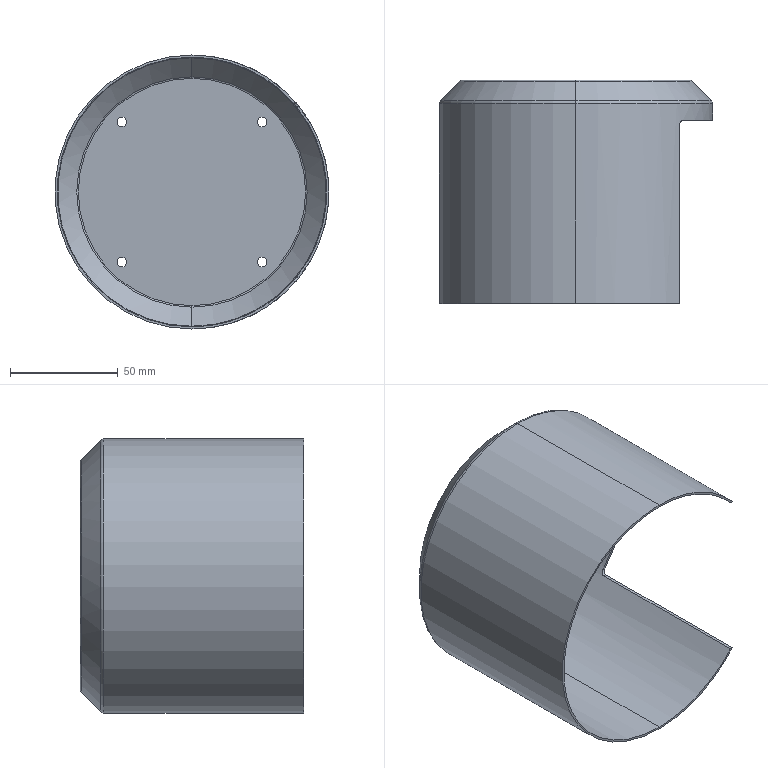Part | SolidWorks | features Fillet 2, Chamfer 1, Extrusion 1, HoleWzd 1, ICE 1, Shell 1 | 1 solid | 32 faces | box 127 x 103.5 x 127 mm | volume 43057 mm3 | cylinder 14 | torus 8 | plane 6 | cone 4 | commonest cylinder face diameters 4.5 x8 4 x2 125 x2 127 x2
STEP:
#1=CARTESIAN_POINT('',(-32.5,50.75,-34.75));
#2=VERTEX_POINT('',#1);
#3=CARTESIAN_POINT('',(-32.5,50.75,-30.25));
#4=VERTEX_POINT('',#3);
#5=CARTESIAN_POINT('',(-32.5,50.75,-32.5));
#6=DIRECTION('',(0.,1.,0.));
#7=DIRECTION('',(0.,0.,1.));
#8=AXIS2_PLACEMENT_3D('',#5,#6,#7);
#9=CIRCLE('',#8,2.25);
#10=EDGE_CURVE('',#2,#4,#9,.T.);
#11=ORIENTED_EDGE('',*,*,#10,.F.);
#12=CARTESIAN_POINT('',(-32.5,51.75,-34.75));
#13=VERTEX_POINT('',#12);
#14=CARTESIAN_POINT('',(-32.5,51.75,-34.75));
#15=DIRECTION('',(0.,1.,0.));
#16=VECTOR('',#15,1000.);
#17=LINE('',#14,#16);
#18=EDGE_CURVE('',#2,#13,#17,.T.);
#19=ORIENTED_EDGE('',*,*,#18,.T.);
#20=CARTESIAN_POINT('',(-32.5,51.75,-30.25));
#21=VERTEX_POINT('',#20);
#22=CARTESIAN_POINT('',(-32.5,51.75,-32.5));
#23=DIRECTION('',(0.,1.,0.));
#24=DIRECTION('',(0.,0.,1.));
#25=AXIS2_PLACEMENT_3D('',#22,#23,#24);
#26=CIRCLE('',#25,2.25);
#27=EDGE_CURVE('',#13,#21,#26,.T.);
#28=ORIENTED_EDGE('',*,*,#27,.T.);
#29=CARTESIAN_POINT('',(-32.5,51.75,-30.25));
#30=DIRECTION('',(0.,1.,0.));
#31=VECTOR('',#30,1000.);
#32=LINE('',#29,#31);
#33=EDGE_CURVE('',#4,#21,#32,.T.);
#34=ORIENTED_EDGE('',*,*,#33,.F.);
#35=EDGE_LOOP('',(#11,#19,#28,#34));
#36=FACE_OUTER_BOUND('',#35,.T.);
#37=CARTESIAN_POINT('',(-32.5,51.75,-32.5));
#38=DIRECTION('',(0.,1.,0.));
#39=DIRECTION('',(0.,0.,1.));
#40=AXIS2_PLACEMENT_3D('',#37,#38,#39);
#41=CYLINDRICAL_SURFACE('',#40,2.25);
#42=ADVANCED_FACE('',(#36),#41,.F.);
#43=CARTESIAN_POINT('',(32.5,50.75,-34.75));
#44=VERTEX_POINT('',#43);
#45=CARTESIAN_POINT('',(32.5,50.75,-30.25));
#46=VERTEX_POINT('',#45);
#47=CARTESIAN_POINT('',(32.5,50.75,-32.5));
#48=DIRECTION('',(0.,1.,0.));
#49=DIRECTION('',(0.,0.,1.));
#50=AXIS2_PLACEMENT_3D('',#47,#48,#49);
#51=CIRCLE('',#50,2.25);
#52=EDGE_CURVE('',#44,#46,#51,.T.);
#53=ORIENTED_EDGE('',*,*,#52,.F.);
#54=CARTESIAN_POINT('',(32.5,51.75,-34.75));
#55=VERTEX_POINT('',#54);
#56=CARTESIAN_POINT('',(32.5,51.75,-34.75));
#57=DIRECTION('',(0.,1.,0.));
#58=VECTOR('',#57,1000.);
#59=LINE('',#56,#58);
#60=EDGE_CURVE('',#44,#55,#59,.T.);
#61=ORIENTED_EDGE('',*,*,#60,.T.);
#62=CARTESIAN_POINT('',(32.5,51.75,-30.25));
#63=VERTEX_POINT('',#62);
#64=CARTESIAN_POINT('',(32.5,51.75,-32.5));
#65=DIRECTION('',(0.,1.,0.));
#66=DIRECTION('',(0.,0.,1.));
#67=AXIS2_PLACEMENT_3D('',#64,#65,#66);
#68=CIRCLE('',#67,2.25);
#69=EDGE_CURVE('',#55,#63,#68,.T.);
#70=ORIENTED_EDGE('',*,*,#69,.T.);
#71=CARTESIAN_POINT('',(32.5,51.75,-30.25));
#72=DIRECTION('',(0.,1.,0.));
#73=VECTOR('',#72,1000.);
#74=LINE('',#71,#73);
#75=EDGE_CURVE('',#46,#63,#74,.T.);
#76=ORIENTED_EDGE('',*,*,#75,.F.);
#77=EDGE_LOOP('',(#53,#61,#70,#76));
#78=FACE_OUTER_BOUND('',#77,.T.);
#79=CARTESIAN_POINT('',(32.5,51.75,-32.5));
#80=DIRECTION('',(0.,1.,0.));
#81=DIRECTION('',(0.,0.,1.));
#82=AXIS2_PLACEMENT_3D('',#79,#80,#81);
#83=CYLINDRICAL_SURFACE('',#82,2.25);
#84=ADVANCED_FACE('',(#78),#83,.F.);
#85=CARTESIAN_POINT('',(32.5,50.75,30.25));
#86=VERTEX_POINT('',#85);
#87=CARTESIAN_POINT('',(32.5,50.75,34.75));
#88=VERTEX_POINT('',#87);
#89=CARTESIAN_POINT('',(32.5,50.75,32.5));
#90=DIRECTION('',(0.,1.,0.));
#91=DIRECTION('',(0.,0.,1.));
#92=AXIS2_PLACEMENT_3D('',#89,#90,#91);
#93=CIRCLE('',#92,2.25);
#94=EDGE_CURVE('',#86,#88,#93,.T.);
#95=ORIENTED_EDGE('',*,*,#94,.F.);
#96=CARTESIAN_POINT('',(32.5,51.75,30.25));
#97=VERTEX_POINT('',#96);
#98=CARTESIAN_POINT('',(32.5,51.75,30.25));
#99=DIRECTION('',(0.,1.,0.));
#100=VECTOR('',#99,1000.);
#101=LINE('',#98,#100);
#102=EDGE_CURVE('',#86,#97,#101,.T.);
#103=ORIENTED_EDGE('',*,*,#102,.T.);
#104=CARTESIAN_POINT('',(32.5,51.75,34.75));
#105=VERTEX_POINT('',#104);
#106=CARTESIAN_POINT('',(32.5,51.75,32.5));
#107=DIRECTION('',(0.,1.,0.));
#108=DIRECTION('',(0.,0.,1.));
#109=AXIS2_PLACEMENT_3D('',#106,#107,#108);
#110=CIRCLE('',#109,2.25);
#111=EDGE_CURVE('',#97,#105,#110,.T.);
#112=ORIENTED_EDGE('',*,*,#111,.T.);
#113=CARTESIAN_POINT('',(32.5,51.75,34.75));
#114=DIRECTION('',(0.,1.,0.));
#115=VECTOR('',#114,1000.);
#116=LINE('',#113,#115);
#117=EDGE_CURVE('',#88,#105,#116,.T.);
#118=ORIENTED_EDGE('',*,*,#117,.F.);
#119=EDGE_LOOP('',(#95,#103,#112,#118));
#120=FACE_OUTER_BOUND('',#119,.T.);
#121=CARTESIAN_POINT('',(32.5,51.75,32.5));
#122=DIRECTION('',(0.,1.,0.));
#123=DIRECTION('',(0.,0.,1.));
#124=AXIS2_PLACEMENT_3D('',#121,#122,#123);
#125=CYLINDRICAL_SURFACE('',#124,2.25);
#126=ADVANCED_FACE('',(#120),#125,.F.);
#127=CARTESIAN_POINT('',(-32.5,50.75,30.25));
#128=VERTEX_POINT('',#127);
#129=CARTESIAN_POINT('',(-32.5,50.75,34.75));
#130=VERTEX_POINT('',#129);
#131=CARTESIAN_POINT('',(-32.5,50.75,32.5));
#132=DIRECTION('',(0.,1.,0.));
#133=DIRECTION('',(0.,0.,1.));
#134=AXIS2_PLACEMENT_3D('',#131,#132,#133);
#135=CIRCLE('',#134,2.25);
#136=EDGE_CURVE('',#128,#130,#135,.T.);
#137=ORIENTED_EDGE('',*,*,#136,.F.);
#138=CARTESIAN_POINT('',(-32.5,51.75,30.25));
#139=VERTEX_POINT('',#138);
#140=CARTESIAN_POINT('',(-32.5,51.75,30.25));
#141=DIRECTION('',(0.,1.,0.));
#142=VECTOR('',#141,1000.);
#143=LINE('',#140,#142);
#144=EDGE_CURVE('',#128,#139,#143,.T.);
#145=ORIENTED_EDGE('',*,*,#144,.T.);
#146=CARTESIAN_POINT('',(-32.5,51.75,34.75));
#147=VERTEX_POINT('',#146);
#148=CARTESIAN_POINT('',(-32.5,51.75,32.5));
#149=DIRECTION('',(0.,1.,0.));
#150=DIRECTION('',(0.,0.,1.));
#151=AXIS2_PLACEMENT_3D('',#148,#149,#150);
#152=CIRCLE('',#151,2.25);
#153=EDGE_CURVE('',#139,#147,#152,.T.);
#154=ORIENTED_EDGE('',*,*,#153,.T.);
#155=CARTESIAN_POINT('',(-32.5,51.75,34.75));
#156=DIRECTION('',(0.,1.,0.));
#157=VECTOR('',#156,1000.);
#158=LINE('',#155,#157);
#159=EDGE_CURVE('',#130,#147,#158,.T.);
#160=ORIENTED_EDGE('',*,*,#159,.F.);
#161=EDGE_LOOP('',(#137,#145,#154,#160));
#162=FACE_OUTER_BOUND('',#161,.T.);
#163=CARTESIAN_POINT('',(-32.5,51.75,32.5));
#164=DIRECTION('',(0.,1.,0.));
#165=DIRECTION('',(0.,0.,1.));
#166=AXIS2_PLACEMENT_3D('',#163,#164,#165);
#167=CYLINDRICAL_SURFACE('',#166,2.25);
#168=ADVANCED_FACE('',(#162),#167,.F.);
#169=CARTESIAN_POINT('',(0.,50.457,53.379));
#170=VERTEX_POINT('',#169);
#171=CARTESIAN_POINT('',(0.,50.457,-53.379));
#172=VERTEX_POINT('',#171);
#173=CARTESIAN_POINT('',(0.,50.457,0.));
#174=DIRECTION('',(0.,-1.,0.));
#175=DIRECTION('',(0.,0.,-1.));
#176=AXIS2_PLACEMENT_3D('',#173,#174,#175);
#177=CIRCLE('',#176,53.379);
#178=EDGE_CURVE('',#170,#172,#177,.T.);
#179=ORIENTED_EDGE('',*,*,#178,.T.);
#180=CARTESIAN_POINT('',(0.,50.75,-52.672));
#181=VERTEX_POINT('',#180);
#182=CARTESIAN_POINT('',(0.,49.75,-52.672));
#183=DIRECTION('',(1.,0.,0.));
#184=DIRECTION('',(0.,0.,-1.));
#185=AXIS2_PLACEMENT_3D('',#182,#183,#184);
#186=CIRCLE('',#185,1.);
#187=EDGE_CURVE('',#172,#181,#186,.T.);
#188=ORIENTED_EDGE('',*,*,#187,.T.);
#189=CARTESIAN_POINT('',(0.,50.75,52.672));
#190=VERTEX_POINT('',#189);
#191=CARTESIAN_POINT('',(0.,50.75,0.));
#192=DIRECTION('',(0.,1.,0.));
#193=DIRECTION('',(0.,0.,1.));
#194=AXIS2_PLACEMENT_3D('',#191,#192,#193);
#195=CIRCLE('',#194,52.672);
#196=EDGE_CURVE('',#181,#190,#195,.T.);
#197=ORIENTED_EDGE('',*,*,#196,.T.);
#198=CARTESIAN_POINT('',(0.,49.75,52.672));
#199=DIRECTION('',(-1.,0.,0.));
#200=DIRECTION('',(0.,0.,1.));
#201=AXIS2_PLACEMENT_3D('',#198,#199,#200);
#202=CIRCLE('',#201,1.);
#203=EDGE_CURVE('',#170,#190,#202,.T.);
#204=ORIENTED_EDGE('',*,*,#203,.F.);
#205=EDGE_LOOP('',(#179,#188,#197,#204));
#206=FACE_OUTER_BOUND('',#205,.T.);
#207=CARTESIAN_POINT('',(0.,49.75,0.));
#208=DIRECTION('',(0.,1.,0.));
#209=DIRECTION('',(0.,0.,1.));
#210=AXIS2_PLACEMENT_3D('',#207,#208,#209);
#211=TOROIDAL_SURFACE('',#210,52.672,1.);
#212=ADVANCED_FACE('',(#206),#211,.F.);
#213=CARTESIAN_POINT('',(0.,40.922,62.5));
#214=VERTEX_POINT('',#213);
#215=CARTESIAN_POINT('',(0.,40.922,-62.5));
#216=VERTEX_POINT('',#215);
#217=CARTESIAN_POINT('',(0.,40.922,0.));
#218=DIRECTION('',(0.,-1.,0.));
#219=DIRECTION('',(0.,0.,-1.));
#220=AXIS2_PLACEMENT_3D('',#217,#218,#219);
#221=CIRCLE('',#220,62.5);
#222=EDGE_CURVE('',#214,#216,#221,.T.);
#223=ORIENTED_EDGE('',*,*,#222,.T.);
#224=CARTESIAN_POINT('',(0.,41.629,-62.207));
#225=VERTEX_POINT('',#224);
#226=CARTESIAN_POINT('',(0.,40.922,-61.5));
#227=DIRECTION('',(1.,0.,0.));
#228=DIRECTION('',(0.,0.,-1.));
#229=AXIS2_PLACEMENT_3D('',#226,#227,#228);
#230=CIRCLE('',#229,1.);
#231=EDGE_CURVE('',#216,#225,#230,.T.);
#232=ORIENTED_EDGE('',*,*,#231,.T.);
#233=CARTESIAN_POINT('',(0.,41.629,62.207));
#234=VERTEX_POINT('',#233);
#235=CARTESIAN_POINT('',(0.,41.629,0.));
#236=DIRECTION('',(0.,1.,0.));
#237=DIRECTION('',(0.,0.,-1.));
#238=AXIS2_PLACEMENT_3D('',#235,#236,#237);
#239=CIRCLE('',#238,62.207);
#240=EDGE_CURVE('',#225,#234,#239,.T.);
#241=ORIENTED_EDGE('',*,*,#240,.T.);
#242=CARTESIAN_POINT('',(0.,40.922,61.5));
#243=DIRECTION('',(-1.,0.,0.));
#244=DIRECTION('',(0.,0.,1.));
#245=AXIS2_PLACEMENT_3D('',#242,#243,#244);
#246=CIRCLE('',#245,1.);
#247=EDGE_CURVE('',#214,#234,#246,.T.);
#248=ORIENTED_EDGE('',*,*,#247,.F.);
#249=EDGE_LOOP('',(#223,#232,#241,#248));
#250=FACE_OUTER_BOUND('',#249,.T.);
#251=CARTESIAN_POINT('',(0.,40.922,0.));
#252=DIRECTION('',(0.,1.,0.));
#253=DIRECTION('',(0.,0.,1.));
#254=AXIS2_PLACEMENT_3D('',#251,#252,#253);
#255=TOROIDAL_SURFACE('',#254,61.5,1.);
#256=ADVANCED_FACE('',(#250),#255,.F.);
#257=ORIENTED_EDGE('',*,*,#178,.F.);
#258=CARTESIAN_POINT('',(0.,51.043,52.793));
#259=DIRECTION('',(0.,-0.7071,0.7071));
#260=VECTOR('',#259,1000.);
#261=LINE('',#258,#260);
#262=EDGE_CURVE('',#170,#234,#261,.T.);
#263=ORIENTED_EDGE('',*,*,#262,.T.);
#264=ORIENTED_EDGE('',*,*,#240,.F.);
#265=CARTESIAN_POINT('',(0.,51.043,-52.793));
#266=DIRECTION('',(0.,-0.7071,-0.7071));
#267=VECTOR('',#266,1000.);
#268=LINE('',#265,#267);
#269=EDGE_CURVE('',#172,#225,#268,.T.);
#270=ORIENTED_EDGE('',*,*,#269,.F.);
#271=EDGE_LOOP('',(#257,#263,#264,#270));
#272=FACE_OUTER_BOUND('',#271,.T.);
#273=CARTESIAN_POINT('',(0.,51.043,0.));
#274=DIRECTION('',(0.,-1.,0.));
#275=DIRECTION('',(0.,0.,-1.));
#276=AXIS2_PLACEMENT_3D('',#273,#274,#275);
#277=CONICAL_SURFACE('',#276,52.793,0.7854);
#278=ADVANCED_FACE('',(#272),#277,.F.);
#279=ORIENTED_EDGE('',*,*,#222,.F.);
#280=CARTESIAN_POINT('',(0.,-51.75,62.5));
#281=VERTEX_POINT('',#280);
#282=CARTESIAN_POINT('',(0.,51.75,62.5));
#283=DIRECTION('',(0.,-1.,0.));
#284=VECTOR('',#283,1000.);
#285=LINE('',#282,#284);
#286=EDGE_CURVE('',#214,#281,#285,.T.);
#287=ORIENTED_EDGE('',*,*,#286,.T.);
#288=CARTESIAN_POINT('',(0.,-51.75,-62.5));
#289=VERTEX_POINT('',#288);
#290=CARTESIAN_POINT('',(0.,-51.75,0.));
#291=DIRECTION('',(0.,1.,0.));
#292=DIRECTION('',(0.,0.,1.));
#293=AXIS2_PLACEMENT_3D('',#290,#291,#292);
#294=CIRCLE('',#293,62.5);
#295=EDGE_CURVE('',#289,#281,#294,.T.);
#296=ORIENTED_EDGE('',*,*,#295,.F.);
#297=CARTESIAN_POINT('',(0.,51.75,-62.5));
#298=DIRECTION('',(0.,-1.,0.));
#299=VECTOR('',#298,1000.);
#300=LINE('',#297,#299);
#301=EDGE_CURVE('',#216,#289,#300,.T.);
#302=ORIENTED_EDGE('',*,*,#301,.F.);
#303=EDGE_LOOP('',(#279,#287,#296,#302));
#304=FACE_OUTER_BOUND('',#303,.T.);
#305=CARTESIAN_POINT('',(0.,51.75,0.));
#306=DIRECTION('',(0.,-1.,0.));
#307=DIRECTION('',(0.,0.,-1.));
#308=AXIS2_PLACEMENT_3D('',#305,#306,#307);
#309=CYLINDRICAL_SURFACE('',#308,62.5);
#310=ADVANCED_FACE('',(#304),#309,.F.);
#311=CARTESIAN_POINT('',(0.,51.164,-54.086));
#312=VERTEX_POINT('',#311);
#313=CARTESIAN_POINT('',(0.,51.164,54.086));
#314=VERTEX_POINT('',#313);
#315=CARTESIAN_POINT('',(0.,51.164,0.));
#316=DIRECTION('',(0.,-1.,0.));
#317=DIRECTION('',(0.,0.,1.));
#318=AXIS2_PLACEMENT_3D('',#315,#316,#317);
#319=CIRCLE('',#318,54.086);
#320=EDGE_CURVE('',#312,#314,#319,.T.);
#321=ORIENTED_EDGE('',*,*,#320,.F.);
#322=CARTESIAN_POINT('',(0.,51.75,-52.672));
#323=VERTEX_POINT('',#322);
#324=CARTESIAN_POINT('',(0.,49.75,-52.672));
#325=DIRECTION('',(1.,0.,0.));
#326=DIRECTION('',(0.,0.,-1.));
#327=AXIS2_PLACEMENT_3D('',#324,#325,#326);
#328=CIRCLE('',#327,2.);
#329=EDGE_CURVE('',#312,#323,#328,.T.);
#330=ORIENTED_EDGE('',*,*,#329,.T.);
#331=CARTESIAN_POINT('',(0.,51.75,52.672));
#332=VERTEX_POINT('',#331);
#333=CARTESIAN_POINT('',(0.,51.75,0.));
#334=DIRECTION('',(0.,1.,0.));
#335=DIRECTION('',(0.,0.,1.));
#336=AXIS2_PLACEMENT_3D('',#333,#334,#335);
#337=CIRCLE('',#336,52.672);
#338=EDGE_CURVE('',#332,#323,#337,.T.);
#339=ORIENTED_EDGE('',*,*,#338,.F.);
#340=CARTESIAN_POINT('',(0.,49.75,52.672));
#341=DIRECTION('',(-1.,0.,0.));
#342=DIRECTION('',(0.,0.,1.));
#343=AXIS2_PLACEMENT_3D('',#340,#341,#342);
#344=CIRCLE('',#343,2.);
#345=EDGE_CURVE('',#314,#332,#344,.T.);
#346=ORIENTED_EDGE('',*,*,#345,.F.);
#347=EDGE_LOOP('',(#321,#330,#339,#346));
#348=FACE_OUTER_BOUND('',#347,.T.);
#349=CARTESIAN_POINT('',(0.,49.75,0.));
#350=DIRECTION('',(0.,1.,0.));
#351=DIRECTION('',(0.,0.,1.));
#352=AXIS2_PLACEMENT_3D('',#349,#350,#351);
#353=TOROIDAL_SURFACE('',#352,52.672,2.);
#354=ADVANCED_FACE('',(#348),#353,.T.);
#355=CARTESIAN_POINT('',(0.,40.922,-63.5));
#356=VERTEX_POINT('',#355);
#357=CARTESIAN_POINT('',(0.,40.922,63.5));
#358=VERTEX_POINT('',#357);
#359=CARTESIAN_POINT('',(0.,40.922,0.));
#360=DIRECTION('',(0.,-1.,0.));
#361=DIRECTION('',(0.,0.,1.));
#362=AXIS2_PLACEMENT_3D('',#359,#360,#361);
#363=CIRCLE('',#362,63.5);
#364=EDGE_CURVE('',#356,#358,#363,.T.);
#365=ORIENTED_EDGE('',*,*,#364,.F.);
#366=CARTESIAN_POINT('',(0.,42.336,-62.914));
#367=VERTEX_POINT('',#366);
#368=CARTESIAN_POINT('',(0.,40.922,-61.5));
#369=DIRECTION('',(1.,0.,0.));
#370=DIRECTION('',(0.,0.,-1.));
#371=AXIS2_PLACEMENT_3D('',#368,#369,#370);
#372=CIRCLE('',#371,2.);
#373=EDGE_CURVE('',#356,#367,#372,.T.);
#374=ORIENTED_EDGE('',*,*,#373,.T.);
#375=CARTESIAN_POINT('',(0.,42.336,62.914));
#376=VERTEX_POINT('',#375);
#377=CARTESIAN_POINT('',(0.,42.336,0.));
#378=DIRECTION('',(0.,1.,0.));
#379=DIRECTION('',(0.,0.,-1.));
#380=AXIS2_PLACEMENT_3D('',#377,#378,#379);
#381=CIRCLE('',#380,62.914);
#382=EDGE_CURVE('',#376,#367,#381,.T.);
#383=ORIENTED_EDGE('',*,*,#382,.F.);
#384=CARTESIAN_POINT('',(0.,40.922,61.5));
#385=DIRECTION('',(-1.,0.,0.));
#386=DIRECTION('',(0.,0.,1.));
#387=AXIS2_PLACEMENT_3D('',#384,#385,#386);
#388=CIRCLE('',#387,2.);
#389=EDGE_CURVE('',#358,#376,#388,.T.);
#390=ORIENTED_EDGE('',*,*,#389,.F.);
#391=EDGE_LOOP('',(#365,#374,#383,#390));
#392=FACE_OUTER_BOUND('',#391,.T.);
#393=CARTESIAN_POINT('',(0.,40.922,0.));
#394=DIRECTION('',(0.,1.,0.));
#395=DIRECTION('',(0.,0.,1.));
#396=AXIS2_PLACEMENT_3D('',#393,#394,#395);
#397=TOROIDAL_SURFACE('',#396,61.5,2.);
#398=ADVANCED_FACE('',(#392),#397,.T.);
#399=ORIENTED_EDGE('',*,*,#320,.T.);
#400=CARTESIAN_POINT('',(0.,51.75,53.5));
#401=DIRECTION('',(0.,-0.7071,0.7071));
#402=VECTOR('',#401,1000.);
#403=LINE('',#400,#402);
#404=EDGE_CURVE('',#314,#376,#403,.T.);
#405=ORIENTED_EDGE('',*,*,#404,.T.);
#406=ORIENTED_EDGE('',*,*,#382,.T.);
#407=CARTESIAN_POINT('',(0.,51.75,-53.5));
#408=DIRECTION('',(0.,-0.7071,-0.7071));
#409=VECTOR('',#408,1000.);
#410=LINE('',#407,#409);
#411=EDGE_CURVE('',#312,#367,#410,.T.);
#412=ORIENTED_EDGE('',*,*,#411,.F.);
#413=EDGE_LOOP('',(#399,#405,#406,#412));
#414=FACE_OUTER_BOUND('',#413,.T.);
#415=CARTESIAN_POINT('',(0.,51.75,0.));
#416=DIRECTION('',(0.,-1.,0.));
#417=DIRECTION('',(0.,0.,-1.));
#418=AXIS2_PLACEMENT_3D('',#415,#416,#417);
#419=CONICAL_SURFACE('',#418,53.5,0.7854);
#420=ADVANCED_FACE('',(#414),#419,.T.);
#421=ORIENTED_EDGE('',*,*,#364,.T.);
#422=CARTESIAN_POINT('',(0.,-51.75,63.5));
#423=VERTEX_POINT('',#422);
#424=CARTESIAN_POINT('',(0.,51.75,63.5));
#425=DIRECTION('',(0.,-1.,0.));
#426=VECTOR('',#425,1000.);
#427=LINE('',#424,#426);
#428=EDGE_CURVE('',#358,#423,#427,.T.);
#429=ORIENTED_EDGE('',*,*,#428,.T.);
#430=CARTESIAN_POINT('',(48.062,-51.75,41.5));
#431=VERTEX_POINT('',#430);
#432=CARTESIAN_POINT('',(0.,-51.75,0.));
#433=DIRECTION('',(0.,1.,0.));
#434=DIRECTION('',(0.,0.,1.));
#435=AXIS2_PLACEMENT_3D('',#432,#433,#434);
#436=CIRCLE('',#435,63.5);
#437=EDGE_CURVE('',#423,#431,#436,.T.);
#438=ORIENTED_EDGE('',*,*,#437,.T.);
#439=CARTESIAN_POINT('',(48.062,31.25,41.5));
#440=VERTEX_POINT('',#439);
#441=CARTESIAN_POINT('',(48.062,51.75,41.5));
#442=DIRECTION('',(0.,1.,0.));
#443=VECTOR('',#442,1000.);
#444=LINE('',#441,#443);
#445=EDGE_CURVE('',#431,#440,#444,.T.);
#446=ORIENTED_EDGE('',*,*,#445,.T.);
#447=CARTESIAN_POINT('',(49.719,33.25,39.5));
#448=VERTEX_POINT('',#447);
#449=CARTESIAN_POINT('',(48.062,31.25,41.5));
#450=CARTESIAN_POINT('',(48.062,31.403,41.5));
#451=CARTESIAN_POINT('',(48.077,31.551,41.483));
#452=CARTESIAN_POINT('',(48.134,31.841,41.416));
#453=CARTESIAN_POINT('',(48.177,31.98,41.367));
#454=CARTESIAN_POINT('',(48.281,32.236,41.246));
#455=CARTESIAN_POINT('',(48.344,32.355,41.172));
#456=CARTESIAN_POINT('',(48.481,32.568,41.01));
#457=CARTESIAN_POINT('',(48.556,32.663,40.921));
#458=CARTESIAN_POINT('',(48.798,32.918,40.633));
#459=CARTESIAN_POINT('',(48.974,33.041,40.421));
#460=CARTESIAN_POINT('',(49.341,33.208,39.972));
#461=CARTESIAN_POINT('',(49.53,33.25,39.738));
#462=CARTESIAN_POINT('',(49.719,33.25,39.5));
#463=B_SPLINE_CURVE_WITH_KNOTS('',3,(#449,#450,#451,#452,#453,#454,#455,#456,#457,#458,#459,#460,#461,#462),.UNSPECIFIED.,.F.,.F.,(4,2,2,2,2,2,4),(0.,0.0004508,0.0009016,0.001352,0.001803,0.002705,0.003606),.UNSPECIFIED.);
#464=EDGE_CURVE('',#440,#448,#463,.T.);
#465=ORIENTED_EDGE('',*,*,#464,.T.);
#466=CARTESIAN_POINT('',(49.719,33.25,-39.5));
#467=VERTEX_POINT('',#466);
#468=CARTESIAN_POINT('',(0.,33.25,0.));
#469=DIRECTION('',(0.,-1.,0.));
#470=DIRECTION('',(0.,0.,-1.));
#471=AXIS2_PLACEMENT_3D('',#468,#469,#470);
#472=CIRCLE('',#471,63.5);
#473=EDGE_CURVE('',#467,#448,#472,.T.);
#474=ORIENTED_EDGE('',*,*,#473,.F.);
#475=CARTESIAN_POINT('',(48.062,31.25,-41.5));
#476=VERTEX_POINT('',#475);
#477=CARTESIAN_POINT('',(49.719,33.25,-39.5));
#478=CARTESIAN_POINT('',(49.53,33.25,-39.738));
#479=CARTESIAN_POINT('',(49.344,33.209,-39.969));
#480=CARTESIAN_POINT('',(49.068,33.084,-40.306));
#481=CARTESIAN_POINT('',(48.977,33.032,-40.416));
#482=CARTESIAN_POINT('',(48.803,32.907,-40.627));
#483=CARTESIAN_POINT('',(48.719,32.834,-40.727));
#484=CARTESIAN_POINT('',(48.478,32.581,-41.015));
#485=CARTESIAN_POINT('',(48.334,32.366,-41.184));
#486=CARTESIAN_POINT('',(48.177,31.981,-41.367));
#487=CARTESIAN_POINT('',(48.135,31.845,-41.415));
#488=CARTESIAN_POINT('',(48.078,31.553,-41.483));
#489=CARTESIAN_POINT('',(48.062,31.403,-41.5));
#490=CARTESIAN_POINT('',(48.062,31.25,-41.5));
#491=B_SPLINE_CURVE_WITH_KNOTS('',3,(#477,#478,#479,#480,#481,#482,#483,#484,#485,#486,#487,#488,#489,#490),.UNSPECIFIED.,.F.,.F.,(4,2,2,2,2,2,4),(0.,0.0008994,0.001349,0.001799,0.002698,0.003148,0.003598),.UNSPECIFIED.);
#492=EDGE_CURVE('',#467,#476,#491,.T.);
#493=ORIENTED_EDGE('',*,*,#492,.T.);
#494=CARTESIAN_POINT('',(48.062,-51.75,-41.5));
#495=VERTEX_POINT('',#494);
#496=CARTESIAN_POINT('',(48.062,51.75,-41.5));
#497=DIRECTION('',(0.,-1.,0.));
#498=VECTOR('',#497,1000.);
#499=LINE('',#496,#498);
#500=EDGE_CURVE('',#476,#495,#499,.T.);
#501=ORIENTED_EDGE('',*,*,#500,.T.);
#502=CARTESIAN_POINT('',(0.,-51.75,-63.5));
#503=VERTEX_POINT('',#502);
#504=CARTESIAN_POINT('',(0.,-51.75,0.));
#505=DIRECTION('',(0.,1.,0.));
#506=DIRECTION('',(0.,0.,1.));
#507=AXIS2_PLACEMENT_3D('',#504,#505,#506);
#508=CIRCLE('',#507,63.5);
#509=EDGE_CURVE('',#495,#503,#508,.T.);
#510=ORIENTED_EDGE('',*,*,#509,.T.);
#511=CARTESIAN_POINT('',(0.,51.75,-63.5));
#512=DIRECTION('',(0.,-1.,0.));
#513=VECTOR('',#512,1000.);
#514=LINE('',#511,#513);
#515=EDGE_CURVE('',#356,#503,#514,.T.);
#516=ORIENTED_EDGE('',*,*,#515,.F.);
#517=EDGE_LOOP('',(#421,#429,#438,#446,#465,#474,#493,#501,#510,#516));
#518=FACE_OUTER_BOUND('',#517,.T.);
#519=CARTESIAN_POINT('',(0.,51.75,0.));
#520=DIRECTION('',(0.,-1.,0.));
#521=DIRECTION('',(0.,0.,-1.));
#522=AXIS2_PLACEMENT_3D('',#519,#520,#521);
#523=CYLINDRICAL_SURFACE('',#522,63.5);
#524=ADVANCED_FACE('',(#518),#523,.T.);
#525=ORIENTED_EDGE('',*,*,#428,.F.);
#526=CARTESIAN_POINT('',(0.,40.922,0.));
#527=DIRECTION('',(0.,-1.,0.));
#528=DIRECTION('',(0.,0.,1.));
#529=AXIS2_PLACEMENT_3D('',#526,#527,#528);
#530=CIRCLE('',#529,63.5);
#531=EDGE_CURVE('',#358,#356,#530,.T.);
#532=ORIENTED_EDGE('',*,*,#531,.T.);
#533=ORIENTED_EDGE('',*,*,#515,.T.);
#534=CARTESIAN_POINT('',(0.,-51.75,0.));
#535=DIRECTION('',(0.,1.,0.));
#536=DIRECTION('',(0.,0.,1.));
#537=AXIS2_PLACEMENT_3D('',#534,#535,#536);
#538=CIRCLE('',#537,63.5);
#539=EDGE_CURVE('',#503,#423,#538,.T.);
#540=ORIENTED_EDGE('',*,*,#539,.T.);
#541=EDGE_LOOP('',(#525,#532,#533,#540));
#542=FACE_OUTER_BOUND('',#541,.T.);
#543=CARTESIAN_POINT('',(0.,51.75,0.));
#544=DIRECTION('',(0.,-1.,0.));
#545=DIRECTION('',(0.,0.,-1.));
#546=AXIS2_PLACEMENT_3D('',#543,#544,#545);
#547=CYLINDRICAL_SURFACE('',#546,63.5);
#548=ADVANCED_FACE('',(#542),#547,.T.);
#549=CARTESIAN_POINT('',(-32.5,51.75,-32.5));
#550=DIRECTION('',(0.,1.,0.));
#551=DIRECTION('',(0.,0.,1.));
#552=AXIS2_PLACEMENT_3D('',#549,#550,#551);
#553=CIRCLE('',#552,2.25);
#554=EDGE_CURVE('',#21,#13,#553,.T.);
#555=ORIENTED_EDGE('',*,*,#554,.F.);
#556=ORIENTED_EDGE('',*,*,#27,.F.);
#557=EDGE_LOOP('',(#555,#556));
#558=FACE_BOUND('',#557,.T.);
#559=CARTESIAN_POINT('',(32.5,51.75,-32.5));
#560=DIRECTION('',(0.,1.,0.));
#561=DIRECTION('',(0.,0.,1.));
#562=AXIS2_PLACEMENT_3D('',#559,#560,#561);
#563=CIRCLE('',#562,2.25);
#564=EDGE_CURVE('',#63,#55,#563,.T.);
#565=ORIENTED_EDGE('',*,*,#564,.F.);
#566=ORIENTED_EDGE('',*,*,#69,.F.);
#567=EDGE_LOOP('',(#565,#566));
#568=FACE_BOUND('',#567,.T.);
#569=CARTESIAN_POINT('',(32.5,51.75,32.5));
#570=DIRECTION('',(0.,1.,0.));
#571=DIRECTION('',(0.,0.,1.));
#572=AXIS2_PLACEMENT_3D('',#569,#570,#571);
#573=CIRCLE('',#572,2.25);
#574=EDGE_CURVE('',#105,#97,#573,.T.);
#575=ORIENTED_EDGE('',*,*,#574,.F.);
#576=ORIENTED_EDGE('',*,*,#111,.F.);
#577=EDGE_LOOP('',(#575,#576));
#578=FACE_BOUND('',#577,.T.);
#579=CARTESIAN_POINT('',(-32.5,51.75,32.5));
#580=DIRECTION('',(0.,1.,0.));
#581=DIRECTION('',(0.,0.,1.));
#582=AXIS2_PLACEMENT_3D('',#579,#580,#581);
#583=CIRCLE('',#582,2.25);
#584=EDGE_CURVE('',#147,#139,#583,.T.);
#585=ORIENTED_EDGE('',*,*,#584,.F.);
#586=ORIENTED_EDGE('',*,*,#153,.F.);
#587=EDGE_LOOP('',(#585,#586));
#588=FACE_BOUND('',#587,.T.);
#589=ORIENTED_EDGE('',*,*,#338,.T.);
#590=CARTESIAN_POINT('',(0.,51.75,0.));
#591=DIRECTION('',(0.,1.,0.));
#592=DIRECTION('',(0.,0.,1.));
#593=AXIS2_PLACEMENT_3D('',#590,#591,#592);
#594=CIRCLE('',#593,52.672);
#595=EDGE_CURVE('',#323,#332,#594,.T.);
#596=ORIENTED_EDGE('',*,*,#595,.T.);
#597=EDGE_LOOP('',(#589,#596));
#598=FACE_OUTER_BOUND('',#597,.T.);
#599=CARTESIAN_POINT('',(0.,51.75,0.));
#600=DIRECTION('',(0.,1.,0.));
#601=DIRECTION('',(0.,0.,1.));
#602=AXIS2_PLACEMENT_3D('',#599,#600,#601);
#603=PLANE('',#602);
#604=ADVANCED_FACE('',(#558,#568,#578,#588,#598),#603,.T.);
#605=ORIENTED_EDGE('',*,*,#509,.F.);
#606=CARTESIAN_POINT('',(46.733,-51.75,-41.5));
#607=VERTEX_POINT('',#606);
#608=CARTESIAN_POINT('',(-5.,-51.75,-41.5));
#609=DIRECTION('',(1.,0.,0.));
#610=VECTOR('',#609,1000.);
#611=LINE('',#608,#610);
#612=EDGE_CURVE('',#607,#495,#611,.T.);
#613=ORIENTED_EDGE('',*,*,#612,.F.);
#614=CARTESIAN_POINT('',(0.,-51.75,0.));
#615=DIRECTION('',(0.,1.,0.));
#616=DIRECTION('',(0.,0.,1.));
#617=AXIS2_PLACEMENT_3D('',#614,#615,#616);
#618=CIRCLE('',#617,62.5);
#619=EDGE_CURVE('',#607,#289,#618,.T.);
#620=ORIENTED_EDGE('',*,*,#619,.T.);
#621=ORIENTED_EDGE('',*,*,#295,.T.);
#622=CARTESIAN_POINT('',(46.733,-51.75,41.5));
#623=VERTEX_POINT('',#622);
#624=CARTESIAN_POINT('',(0.,-51.75,0.));
#625=DIRECTION('',(0.,1.,0.));
#626=DIRECTION('',(0.,0.,1.));
#627=AXIS2_PLACEMENT_3D('',#624,#625,#626);
#628=CIRCLE('',#627,62.5);
#629=EDGE_CURVE('',#281,#623,#628,.T.);
#630=ORIENTED_EDGE('',*,*,#629,.T.);
#631=CARTESIAN_POINT('',(-5.,-51.75,41.5));
#632=DIRECTION('',(-1.,0.,0.));
#633=VECTOR('',#632,1000.);
#634=LINE('',#631,#633);
#635=EDGE_CURVE('',#431,#623,#634,.T.);
#636=ORIENTED_EDGE('',*,*,#635,.F.);
#637=ORIENTED_EDGE('',*,*,#437,.F.);
#638=ORIENTED_EDGE('',*,*,#539,.F.);
#639=EDGE_LOOP('',(#605,#613,#620,#621,#630,#636,#637,#638));
#640=FACE_OUTER_BOUND('',#639,.T.);
#641=CARTESIAN_POINT('',(0.,-51.75,0.));
#642=DIRECTION('',(0.,1.,0.));
#643=DIRECTION('',(0.,0.,1.));
#644=AXIS2_PLACEMENT_3D('',#641,#642,#643);
#645=PLANE('',#644);
#646=ADVANCED_FACE('',(#640),#645,.F.);
#647=ORIENTED_EDGE('',*,*,#404,.F.);
#648=CARTESIAN_POINT('',(0.,51.164,0.));
#649=DIRECTION('',(0.,-1.,0.));
#650=DIRECTION('',(0.,0.,1.));
#651=AXIS2_PLACEMENT_3D('',#648,#649,#650);
#652=CIRCLE('',#651,54.086);
#653=EDGE_CURVE('',#314,#312,#652,.T.);
#654=ORIENTED_EDGE('',*,*,#653,.T.);
#655=ORIENTED_EDGE('',*,*,#411,.T.);
#656=CARTESIAN_POINT('',(0.,42.336,0.));
#657=DIRECTION('',(0.,1.,0.));
#658=DIRECTION('',(0.,0.,-1.));
#659=AXIS2_PLACEMENT_3D('',#656,#657,#658);
#660=CIRCLE('',#659,62.914);
#661=EDGE_CURVE('',#367,#376,#660,.T.);
#662=ORIENTED_EDGE('',*,*,#661,.T.);
#663=EDGE_LOOP('',(#647,#654,#655,#662));
#664=FACE_OUTER_BOUND('',#663,.T.);
#665=CARTESIAN_POINT('',(0.,51.75,0.));
#666=DIRECTION('',(0.,-1.,0.));
#667=DIRECTION('',(0.,0.,-1.));
#668=AXIS2_PLACEMENT_3D('',#665,#666,#667);
#669=CONICAL_SURFACE('',#668,53.5,0.7854);
#670=ADVANCED_FACE('',(#664),#669,.T.);
#671=ORIENTED_EDGE('',*,*,#373,.F.);
#672=ORIENTED_EDGE('',*,*,#531,.F.);
#673=ORIENTED_EDGE('',*,*,#389,.T.);
#674=ORIENTED_EDGE('',*,*,#661,.F.);
#675=EDGE_LOOP('',(#671,#672,#673,#674));
#676=FACE_OUTER_BOUND('',#675,.T.);
#677=CARTESIAN_POINT('',(0.,40.922,0.));
#678=DIRECTION('',(0.,1.,0.));
#679=DIRECTION('',(0.,0.,1.));
#680=AXIS2_PLACEMENT_3D('',#677,#678,#679);
#681=TOROIDAL_SURFACE('',#680,61.5,2.);
#682=ADVANCED_FACE('',(#676),#681,.T.);
#683=ORIENTED_EDGE('',*,*,#329,.F.);
#684=ORIENTED_EDGE('',*,*,#653,.F.);
#685=ORIENTED_EDGE('',*,*,#345,.T.);
#686=ORIENTED_EDGE('',*,*,#595,.F.);
#687=EDGE_LOOP('',(#683,#684,#685,#686));
#688=FACE_OUTER_BOUND('',#687,.T.);
#689=CARTESIAN_POINT('',(0.,49.75,0.));
#690=DIRECTION('',(0.,1.,0.));
#691=DIRECTION('',(0.,0.,1.));
#692=AXIS2_PLACEMENT_3D('',#689,#690,#691);
#693=TOROIDAL_SURFACE('',#692,52.672,2.);
#694=ADVANCED_FACE('',(#688),#693,.T.);
#695=ORIENTED_EDGE('',*,*,#286,.F.);
#696=CARTESIAN_POINT('',(0.,40.922,0.));
#697=DIRECTION('',(0.,-1.,0.));
#698=DIRECTION('',(0.,0.,-1.));
#699=AXIS2_PLACEMENT_3D('',#696,#697,#698);
#700=CIRCLE('',#699,62.5);
#701=EDGE_CURVE('',#216,#214,#700,.T.);
#702=ORIENTED_EDGE('',*,*,#701,.F.);
#703=ORIENTED_EDGE('',*,*,#301,.T.);
#704=ORIENTED_EDGE('',*,*,#619,.F.);
#705=CARTESIAN_POINT('',(46.733,31.25,-41.5));
#706=VERTEX_POINT('',#705);
#707=CARTESIAN_POINT('',(46.733,51.75,-41.5));
#708=DIRECTION('',(0.,-1.,0.));
#709=VECTOR('',#708,1000.);
#710=LINE('',#707,#709);
#711=EDGE_CURVE('',#706,#607,#710,.T.);
#712=ORIENTED_EDGE('',*,*,#711,.F.);
#713=CARTESIAN_POINT('',(48.436,33.25,-39.5));
#714=VERTEX_POINT('',#713);
#715=CARTESIAN_POINT('',(46.733,31.25,-41.5));
#716=CARTESIAN_POINT('',(46.733,31.404,-41.5));
#717=CARTESIAN_POINT('',(46.749,31.553,-41.482));
#718=CARTESIAN_POINT('',(46.808,31.844,-41.415));
#719=CARTESIAN_POINT('',(46.852,31.984,-41.366));
#720=CARTESIAN_POINT('',(46.96,32.24,-41.243));
#721=CARTESIAN_POINT('',(47.025,32.359,-41.169));
#722=CARTESIAN_POINT('',(47.167,32.572,-41.007));
#723=CARTESIAN_POINT('',(47.244,32.667,-40.918));
#724=CARTESIAN_POINT('',(47.493,32.921,-40.629));
#725=CARTESIAN_POINT('',(47.673,33.043,-40.418));
#726=CARTESIAN_POINT('',(48.049,33.209,-39.97));
#727=CARTESIAN_POINT('',(48.242,33.25,-39.737));
#728=CARTESIAN_POINT('',(48.436,33.25,-39.5));
#729=B_SPLINE_CURVE_WITH_KNOTS('',3,(#715,#716,#717,#718,#719,#720,#721,#722,#723,#724,#725,#726,#727,#728),.UNSPECIFIED.,.F.,.F.,(4,2,2,2,2,2,4),(0.,0.0004538,0.0009076,0.001361,0.001815,0.002723,0.00363),.UNSPECIFIED.);
#730=EDGE_CURVE('',#706,#714,#729,.T.);
#731=ORIENTED_EDGE('',*,*,#730,.T.);
#732=CARTESIAN_POINT('',(48.436,33.25,39.5));
#733=VERTEX_POINT('',#732);
#734=CARTESIAN_POINT('',(0.,33.25,0.));
#735=DIRECTION('',(0.,-1.,0.));
#736=DIRECTION('',(0.,0.,-1.));
#737=AXIS2_PLACEMENT_3D('',#734,#735,#736);
#738=CIRCLE('',#737,62.5);
#739=EDGE_CURVE('',#714,#733,#738,.T.);
#740=ORIENTED_EDGE('',*,*,#739,.T.);
#741=CARTESIAN_POINT('',(46.733,31.25,41.5));
#742=VERTEX_POINT('',#741);
#743=CARTESIAN_POINT('',(48.436,33.25,39.5));
#744=CARTESIAN_POINT('',(48.242,33.25,39.737));
#745=CARTESIAN_POINT('',(48.052,33.209,39.967));
#746=CARTESIAN_POINT('',(47.769,33.085,40.304));
#747=CARTESIAN_POINT('',(47.676,33.033,40.413));
#748=CARTESIAN_POINT('',(47.498,32.909,40.623));
#749=CARTESIAN_POINT('',(47.411,32.837,40.724));
#750=CARTESIAN_POINT('',(47.163,32.584,41.011));
#751=CARTESIAN_POINT('',(47.015,32.371,41.181));
#752=CARTESIAN_POINT('',(46.852,31.985,41.366));
#753=CARTESIAN_POINT('',(46.809,31.848,41.414));
#754=CARTESIAN_POINT('',(46.749,31.555,41.482));
#755=CARTESIAN_POINT('',(46.733,31.404,41.5));
#756=CARTESIAN_POINT('',(46.733,31.25,41.5));
#757=B_SPLINE_CURVE_WITH_KNOTS('',3,(#743,#744,#745,#746,#747,#748,#749,#750,#751,#752,#753,#754,#755,#756),.UNSPECIFIED.,.F.,.F.,(4,2,2,2,2,2,4),(0.,0.0009058,0.001359,0.001812,0.002717,0.00317,0.003623),.UNSPECIFIED.);
#758=EDGE_CURVE('',#733,#742,#757,.T.);
#759=ORIENTED_EDGE('',*,*,#758,.T.);
#760=CARTESIAN_POINT('',(46.733,51.75,41.5));
#761=DIRECTION('',(0.,1.,0.));
#762=VECTOR('',#761,1000.);
#763=LINE('',#760,#762);
#764=EDGE_CURVE('',#623,#742,#763,.T.);
#765=ORIENTED_EDGE('',*,*,#764,.F.);
#766=ORIENTED_EDGE('',*,*,#629,.F.);
#767=EDGE_LOOP('',(#695,#702,#703,#704,#712,#731,#740,#759,#765,#766));
#768=FACE_OUTER_BOUND('',#767,.T.);
#769=CARTESIAN_POINT('',(0.,51.75,0.));
#770=DIRECTION('',(0.,-1.,0.));
#771=DIRECTION('',(0.,0.,-1.));
#772=AXIS2_PLACEMENT_3D('',#769,#770,#771);
#773=CYLINDRICAL_SURFACE('',#772,62.5);
#774=ADVANCED_FACE('',(#768),#773,.F.);
#775=CARTESIAN_POINT('',(-32.5,50.75,-32.5));
#776=DIRECTION('',(0.,1.,0.));
#777=DIRECTION('',(0.,0.,1.));
#778=AXIS2_PLACEMENT_3D('',#775,#776,#777);
#779=CIRCLE('',#778,2.25);
#780=EDGE_CURVE('',#4,#2,#779,.T.);
#781=ORIENTED_EDGE('',*,*,#780,.T.);
#782=ORIENTED_EDGE('',*,*,#10,.T.);
#783=EDGE_LOOP('',(#781,#782));
#784=FACE_BOUND('',#783,.T.);
#785=CARTESIAN_POINT('',(32.5,50.75,-32.5));
#786=DIRECTION('',(0.,1.,0.));
#787=DIRECTION('',(0.,0.,1.));
#788=AXIS2_PLACEMENT_3D('',#785,#786,#787);
#789=CIRCLE('',#788,2.25);
#790=EDGE_CURVE('',#46,#44,#789,.T.);
#791=ORIENTED_EDGE('',*,*,#790,.T.);
#792=ORIENTED_EDGE('',*,*,#52,.T.);
#793=EDGE_LOOP('',(#791,#792));
#794=FACE_BOUND('',#793,.T.);
#795=CARTESIAN_POINT('',(32.5,50.75,32.5));
#796=DIRECTION('',(0.,1.,0.));
#797=DIRECTION('',(0.,0.,1.));
#798=AXIS2_PLACEMENT_3D('',#795,#796,#797);
#799=CIRCLE('',#798,2.25);
#800=EDGE_CURVE('',#88,#86,#799,.T.);
#801=ORIENTED_EDGE('',*,*,#800,.T.);
#802=ORIENTED_EDGE('',*,*,#94,.T.);
#803=EDGE_LOOP('',(#801,#802));
#804=FACE_BOUND('',#803,.T.);
#805=CARTESIAN_POINT('',(-32.5,50.75,32.5));
#806=DIRECTION('',(0.,1.,0.));
#807=DIRECTION('',(0.,0.,1.));
#808=AXIS2_PLACEMENT_3D('',#805,#806,#807);
#809=CIRCLE('',#808,2.25);
#810=EDGE_CURVE('',#130,#128,#809,.T.);
#811=ORIENTED_EDGE('',*,*,#810,.T.);
#812=ORIENTED_EDGE('',*,*,#136,.T.);
#813=EDGE_LOOP('',(#811,#812));
#814=FACE_BOUND('',#813,.T.);
#815=CARTESIAN_POINT('',(0.,50.75,0.));
#816=DIRECTION('',(0.,1.,0.));
#817=DIRECTION('',(0.,0.,1.));
#818=AXIS2_PLACEMENT_3D('',#815,#816,#817);
#819=CIRCLE('',#818,52.672);
#820=EDGE_CURVE('',#190,#181,#819,.T.);
#821=ORIENTED_EDGE('',*,*,#820,.F.);
#822=ORIENTED_EDGE('',*,*,#196,.F.);
#823=EDGE_LOOP('',(#821,#822));
#824=FACE_OUTER_BOUND('',#823,.T.);
#825=CARTESIAN_POINT('',(0.,50.75,0.));
#826=DIRECTION('',(0.,1.,0.));
#827=DIRECTION('',(0.,0.,1.));
#828=AXIS2_PLACEMENT_3D('',#825,#826,#827);
#829=PLANE('',#828);
#830=ADVANCED_FACE('',(#784,#794,#804,#814,#824),#829,.F.);
#831=ORIENTED_EDGE('',*,*,#262,.F.);
#832=CARTESIAN_POINT('',(0.,50.457,0.));
#833=DIRECTION('',(0.,-1.,0.));
#834=DIRECTION('',(0.,0.,-1.));
#835=AXIS2_PLACEMENT_3D('',#832,#833,#834);
#836=CIRCLE('',#835,53.379);
#837=EDGE_CURVE('',#172,#170,#836,.T.);
#838=ORIENTED_EDGE('',*,*,#837,.F.);
#839=ORIENTED_EDGE('',*,*,#269,.T.);
#840=CARTESIAN_POINT('',(0.,41.629,0.));
#841=DIRECTION('',(0.,1.,0.));
#842=DIRECTION('',(0.,0.,-1.));
#843=AXIS2_PLACEMENT_3D('',#840,#841,#842);
#844=CIRCLE('',#843,62.207);
#845=EDGE_CURVE('',#234,#225,#844,.T.);
#846=ORIENTED_EDGE('',*,*,#845,.F.);
#847=EDGE_LOOP('',(#831,#838,#839,#846));
#848=FACE_OUTER_BOUND('',#847,.T.);
#849=CARTESIAN_POINT('',(0.,51.043,0.));
#850=DIRECTION('',(0.,-1.,0.));
#851=DIRECTION('',(0.,0.,-1.));
#852=AXIS2_PLACEMENT_3D('',#849,#850,#851);
#853=CONICAL_SURFACE('',#852,52.793,0.7854);
#854=ADVANCED_FACE('',(#848),#853,.F.);
#855=ORIENTED_EDGE('',*,*,#231,.F.);
#856=ORIENTED_EDGE('',*,*,#701,.T.);
#857=ORIENTED_EDGE('',*,*,#247,.T.);
#858=ORIENTED_EDGE('',*,*,#845,.T.);
#859=EDGE_LOOP('',(#855,#856,#857,#858));
#860=FACE_OUTER_BOUND('',#859,.T.);
#861=CARTESIAN_POINT('',(0.,40.922,0.));
#862=DIRECTION('',(0.,1.,0.));
#863=DIRECTION('',(0.,0.,1.));
#864=AXIS2_PLACEMENT_3D('',#861,#862,#863);
#865=TOROIDAL_SURFACE('',#864,61.5,1.);
#866=ADVANCED_FACE('',(#860),#865,.F.);
#867=ORIENTED_EDGE('',*,*,#187,.F.);
#868=ORIENTED_EDGE('',*,*,#837,.T.);
#869=ORIENTED_EDGE('',*,*,#203,.T.);
#870=ORIENTED_EDGE('',*,*,#820,.T.);
#871=EDGE_LOOP('',(#867,#868,#869,#870));
#872=FACE_OUTER_BOUND('',#871,.T.);
#873=CARTESIAN_POINT('',(0.,49.75,0.));
#874=DIRECTION('',(0.,1.,0.));
#875=DIRECTION('',(0.,0.,1.));
#876=AXIS2_PLACEMENT_3D('',#873,#874,#875);
#877=TOROIDAL_SURFACE('',#876,52.672,1.);
#878=ADVANCED_FACE('',(#872),#877,.F.);
#879=ORIENTED_EDGE('',*,*,#144,.F.);
#880=ORIENTED_EDGE('',*,*,#810,.F.);
#881=ORIENTED_EDGE('',*,*,#159,.T.);
#882=ORIENTED_EDGE('',*,*,#584,.T.);
#883=EDGE_LOOP('',(#879,#880,#881,#882));
#884=FACE_OUTER_BOUND('',#883,.T.);
#885=CARTESIAN_POINT('',(-32.5,51.75,32.5));
#886=DIRECTION('',(0.,1.,0.));
#887=DIRECTION('',(0.,0.,1.));
#888=AXIS2_PLACEMENT_3D('',#885,#886,#887);
#889=CYLINDRICAL_SURFACE('',#888,2.25);
#890=ADVANCED_FACE('',(#884),#889,.F.);
#891=ORIENTED_EDGE('',*,*,#102,.F.);
#892=ORIENTED_EDGE('',*,*,#800,.F.);
#893=ORIENTED_EDGE('',*,*,#117,.T.);
#894=ORIENTED_EDGE('',*,*,#574,.T.);
#895=EDGE_LOOP('',(#891,#892,#893,#894));
#896=FACE_OUTER_BOUND('',#895,.T.);
#897=CARTESIAN_POINT('',(32.5,51.75,32.5));
#898=DIRECTION('',(0.,1.,0.));
#899=DIRECTION('',(0.,0.,1.));
#900=AXIS2_PLACEMENT_3D('',#897,#898,#899);
#901=CYLINDRICAL_SURFACE('',#900,2.25);
#902=ADVANCED_FACE('',(#896),#901,.F.);
#903=ORIENTED_EDGE('',*,*,#60,.F.);
#904=ORIENTED_EDGE('',*,*,#790,.F.);
#905=ORIENTED_EDGE('',*,*,#75,.T.);
#906=ORIENTED_EDGE('',*,*,#564,.T.);
#907=EDGE_LOOP('',(#903,#904,#905,#906));
#908=FACE_OUTER_BOUND('',#907,.T.);
#909=CARTESIAN_POINT('',(32.5,51.75,-32.5));
#910=DIRECTION('',(0.,1.,0.));
#911=DIRECTION('',(0.,0.,1.));
#912=AXIS2_PLACEMENT_3D('',#909,#910,#911);
#913=CYLINDRICAL_SURFACE('',#912,2.25);
#914=ADVANCED_FACE('',(#908),#913,.F.);
#915=ORIENTED_EDGE('',*,*,#18,.F.);
#916=ORIENTED_EDGE('',*,*,#780,.F.);
#917=ORIENTED_EDGE('',*,*,#33,.T.);
#918=ORIENTED_EDGE('',*,*,#554,.T.);
#919=EDGE_LOOP('',(#915,#916,#917,#918));
#920=FACE_OUTER_BOUND('',#919,.T.);
#921=CARTESIAN_POINT('',(-32.5,51.75,-32.5));
#922=DIRECTION('',(0.,1.,0.));
#923=DIRECTION('',(0.,0.,1.));
#924=AXIS2_PLACEMENT_3D('',#921,#922,#923);
#925=CYLINDRICAL_SURFACE('',#924,2.25);
#926=ADVANCED_FACE('',(#920),#925,.F.);
#927=ORIENTED_EDGE('',*,*,#500,.F.);
#928=CARTESIAN_POINT('',(-5.,31.25,-41.5));
#929=DIRECTION('',(-1.,0.,0.));
#930=VECTOR('',#929,1000.);
#931=LINE('',#928,#930);
#932=EDGE_CURVE('',#476,#706,#931,.T.);
#933=ORIENTED_EDGE('',*,*,#932,.T.);
#934=ORIENTED_EDGE('',*,*,#711,.T.);
#935=ORIENTED_EDGE('',*,*,#612,.T.);
#936=EDGE_LOOP('',(#927,#933,#934,#935));
#937=FACE_OUTER_BOUND('',#936,.T.);
#938=CARTESIAN_POINT('',(-5.,33.25,-41.5));
#939=DIRECTION('',(0.,0.,-1.));
#940=DIRECTION('',(-1.,0.,0.));
#941=AXIS2_PLACEMENT_3D('',#938,#939,#940);
#942=PLANE('',#941);
#943=ADVANCED_FACE('',(#937),#942,.F.);
#944=ORIENTED_EDGE('',*,*,#764,.T.);
#945=CARTESIAN_POINT('',(-5.,31.25,41.5));
#946=DIRECTION('',(1.,0.,0.));
#947=VECTOR('',#946,1000.);
#948=LINE('',#945,#947);
#949=EDGE_CURVE('',#742,#440,#948,.T.);
#950=ORIENTED_EDGE('',*,*,#949,.T.);
#951=ORIENTED_EDGE('',*,*,#445,.F.);
#952=ORIENTED_EDGE('',*,*,#635,.T.);
#953=EDGE_LOOP('',(#944,#950,#951,#952));
#954=FACE_OUTER_BOUND('',#953,.T.);
#955=CARTESIAN_POINT('',(-5.,33.25,41.5));
#956=DIRECTION('',(0.,0.,1.));
#957=DIRECTION('',(1.,0.,0.));
#958=AXIS2_PLACEMENT_3D('',#955,#956,#957);
#959=PLANE('',#958);
#960=ADVANCED_FACE('',(#954),#959,.F.);
#961=ORIENTED_EDGE('',*,*,#473,.T.);
#962=CARTESIAN_POINT('',(0.,33.25,39.5));
#963=DIRECTION('',(-1.,0.,0.));
#964=VECTOR('',#963,1000.);
#965=LINE('',#962,#964);
#966=EDGE_CURVE('',#448,#733,#965,.T.);
#967=ORIENTED_EDGE('',*,*,#966,.T.);
#968=ORIENTED_EDGE('',*,*,#739,.F.);
#969=CARTESIAN_POINT('',(0.,33.25,-39.5));
#970=DIRECTION('',(1.,0.,0.));
#971=VECTOR('',#970,1000.);
#972=LINE('',#969,#971);
#973=EDGE_CURVE('',#714,#467,#972,.T.);
#974=ORIENTED_EDGE('',*,*,#973,.T.);
#975=EDGE_LOOP('',(#961,#967,#968,#974));
#976=FACE_OUTER_BOUND('',#975,.T.);
#977=CARTESIAN_POINT('',(0.,33.25,0.));
#978=DIRECTION('',(0.,-1.,0.));
#979=DIRECTION('',(0.,0.,-1.));
#980=AXIS2_PLACEMENT_3D('',#977,#978,#979);
#981=PLANE('',#980);
#982=ADVANCED_FACE('',(#976),#981,.T.);
#983=ORIENTED_EDGE('',*,*,#464,.F.);
#984=ORIENTED_EDGE('',*,*,#949,.F.);
#985=ORIENTED_EDGE('',*,*,#758,.F.);
#986=ORIENTED_EDGE('',*,*,#966,.F.);
#987=EDGE_LOOP('',(#983,#984,#985,#986));
#988=FACE_OUTER_BOUND('',#987,.T.);
#989=CARTESIAN_POINT('',(0.,31.25,39.5));
#990=DIRECTION('',(-1.,0.,0.));
#991=DIRECTION('',(0.,0.,1.));
#992=AXIS2_PLACEMENT_3D('',#989,#990,#991);
#993=CYLINDRICAL_SURFACE('',#992,2.);
#994=ADVANCED_FACE('',(#988),#993,.F.);
#995=ORIENTED_EDGE('',*,*,#730,.F.);
#996=ORIENTED_EDGE('',*,*,#932,.F.);
#997=ORIENTED_EDGE('',*,*,#492,.F.);
#998=ORIENTED_EDGE('',*,*,#973,.F.);
#999=EDGE_LOOP('',(#995,#996,#997,#998));
#1000=FACE_OUTER_BOUND('',#999,.T.);
#1001=CARTESIAN_POINT('',(0.,31.25,-39.5));
#1002=DIRECTION('',(1.,0.,0.));
#1003=DIRECTION('',(0.,0.,-1.));
#1004=AXIS2_PLACEMENT_3D('',#1001,#1002,#1003);
#1005=CYLINDRICAL_SURFACE('',#1004,2.);
#1006=ADVANCED_FACE('',(#1000),#1005,.F.);
#1007=CLOSED_SHELL('',(#42,#84,#126,#168,#212,#256,#278,#310,#354,#398,#420,#524,#548,#604,#646,#670,#682,#694,#774,#830,#854,#866,#878,#890,#902,#914,#926,#943,#960,#982,#994,#1006));
#1008=MANIFOLD_SOLID_BREP('',#1007);
#1009=CARTESIAN_POINT('',(0.,0.,0.));
#1010=DIRECTION('',(0.,0.,1.));
#1011=DIRECTION('',(1.,0.,0.));
#1012=AXIS2_PLACEMENT_3D('',#1009,#1010,#1011);
#1013=(LENGTH_UNIT()NAMED_UNIT(*)SI_UNIT(.MILLI.,.METRE.));
#1014=UNCERTAINTY_MEASURE_WITH_UNIT(LENGTH_MEASURE(0.00001),#1013,'','');
#1015=(NAMED_UNIT(*)PLANE_ANGLE_UNIT()SI_UNIT($,.RADIAN.));
#1016=(NAMED_UNIT(*)SI_UNIT($,.STERADIAN.)SOLID_ANGLE_UNIT());
#1017=(GEOMETRIC_REPRESENTATION_CONTEXT(3)GLOBAL_UNCERTAINTY_ASSIGNED_CONTEXT((#1014))GLOBAL_UNIT_ASSIGNED_CONTEXT((#1013,#1015,#1016))REPRESENTATION_CONTEXT('',''));
#1018=ADVANCED_BREP_SHAPE_REPRESENTATION('',(#1008,#1012),#1017);